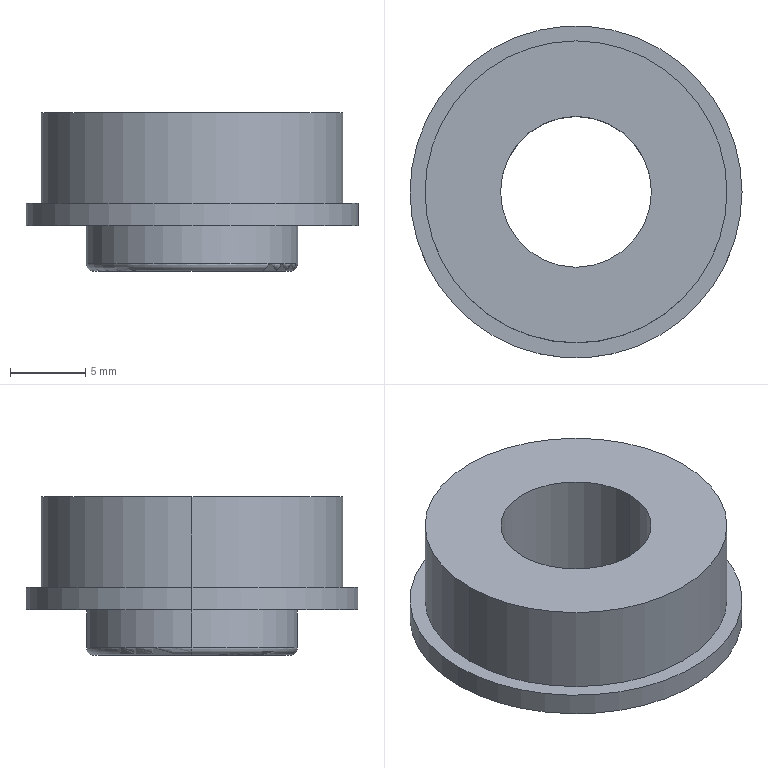Part | 1 solid | 14 faces | box 22 x 22 x 10.5 mm | volume 2090 mm3 | cylinder 8 | plane 4 | torus 2 | commonest cylinder face diameters 10 x2 14 x2 20 x2 22 x2
STEP:
#1=CARTESIAN_POINT('',(5.,0.,10.5));
#2=VERTEX_POINT('',#1);
#3=CARTESIAN_POINT('',(-5.,0.,10.5));
#4=VERTEX_POINT('',#3);
#5=CARTESIAN_POINT('',(0.,0.,10.5));
#6=DIRECTION('',(0.,0.,-1.));
#7=DIRECTION('',(-1.,0.,0.));
#8=AXIS2_PLACEMENT_3D('',#5,#6,#7);
#9=CIRCLE('',#8,5.);
#10=EDGE_CURVE('',#2,#4,#9,.T.);
#11=ORIENTED_EDGE('',*,*,#10,.F.);
#12=CARTESIAN_POINT('',(5.,0.,0.));
#13=VERTEX_POINT('',#12);
#14=CARTESIAN_POINT('',(5.,0.,10.5));
#15=DIRECTION('',(0.,0.,-1.));
#16=VECTOR('',#15,1000.);
#17=LINE('',#14,#16);
#18=EDGE_CURVE('',#2,#13,#17,.T.);
#19=ORIENTED_EDGE('',*,*,#18,.T.);
#20=CARTESIAN_POINT('',(-5.,0.,0.));
#21=VERTEX_POINT('',#20);
#22=CARTESIAN_POINT('',(0.,0.,0.));
#23=DIRECTION('',(0.,0.,-1.));
#24=DIRECTION('',(-1.,0.,0.));
#25=AXIS2_PLACEMENT_3D('',#22,#23,#24);
#26=CIRCLE('',#25,5.);
#27=EDGE_CURVE('',#13,#21,#26,.T.);
#28=ORIENTED_EDGE('',*,*,#27,.T.);
#29=CARTESIAN_POINT('',(-5.,0.,10.5));
#30=DIRECTION('',(0.,0.,-1.));
#31=VECTOR('',#30,1000.);
#32=LINE('',#29,#31);
#33=EDGE_CURVE('',#4,#21,#32,.T.);
#34=ORIENTED_EDGE('',*,*,#33,.F.);
#35=EDGE_LOOP('',(#11,#19,#28,#34));
#36=FACE_OUTER_BOUND('',#35,.T.);
#37=CARTESIAN_POINT('',(0.,0.,10.5));
#38=DIRECTION('',(0.,0.,-1.));
#39=DIRECTION('',(-1.,0.,0.));
#40=AXIS2_PLACEMENT_3D('',#37,#38,#39);
#41=CYLINDRICAL_SURFACE('',#40,5.);
#42=ADVANCED_FACE('',(#36),#41,.F.);
#43=CARTESIAN_POINT('',(-6.5,0.,0.));
#44=VERTEX_POINT('',#43);
#45=CARTESIAN_POINT('',(6.5,0.,0.));
#46=VERTEX_POINT('',#45);
#47=CARTESIAN_POINT('',(0.,0.,0.));
#48=DIRECTION('',(0.,0.,-1.));
#49=DIRECTION('',(1.,0.,0.));
#50=AXIS2_PLACEMENT_3D('',#47,#48,#49);
#51=CIRCLE('',#50,6.5);
#52=EDGE_CURVE('',#44,#46,#51,.T.);
#53=ORIENTED_EDGE('',*,*,#52,.F.);
#54=CARTESIAN_POINT('',(-7.,0.,0.5));
#55=VERTEX_POINT('',#54);
#56=CARTESIAN_POINT('',(-6.5,0.,0.5));
#57=DIRECTION('',(0.,1.,0.));
#58=DIRECTION('',(-1.,0.,0.));
#59=AXIS2_PLACEMENT_3D('',#56,#57,#58);
#60=CIRCLE('',#59,0.5);
#61=EDGE_CURVE('',#44,#55,#60,.T.);
#62=ORIENTED_EDGE('',*,*,#61,.T.);
#63=CARTESIAN_POINT('',(7.,0.,0.5));
#64=VERTEX_POINT('',#63);
#65=CARTESIAN_POINT('',(0.,0.,0.5));
#66=DIRECTION('',(0.,0.,1.));
#67=DIRECTION('',(1.,0.,0.));
#68=AXIS2_PLACEMENT_3D('',#65,#66,#67);
#69=CIRCLE('',#68,7.);
#70=EDGE_CURVE('',#64,#55,#69,.T.);
#71=ORIENTED_EDGE('',*,*,#70,.F.);
#72=CARTESIAN_POINT('',(6.5,0.,0.5));
#73=DIRECTION('',(0.,-1.,0.));
#74=DIRECTION('',(0.,0.,-1.));
#75=AXIS2_PLACEMENT_3D('',#72,#73,#74);
#76=CIRCLE('',#75,0.5);
#77=EDGE_CURVE('',#46,#64,#76,.T.);
#78=ORIENTED_EDGE('',*,*,#77,.F.);
#79=EDGE_LOOP('',(#53,#62,#71,#78));
#80=FACE_OUTER_BOUND('',#79,.T.);
#81=CARTESIAN_POINT('',(0.,0.,0.5));
#82=DIRECTION('',(0.,0.,1.));
#83=DIRECTION('',(1.,0.,0.));
#84=AXIS2_PLACEMENT_3D('',#81,#82,#83);
#85=TOROIDAL_SURFACE('',#84,6.5,0.5);
#86=ADVANCED_FACE('',(#80),#85,.T.);
#87=CARTESIAN_POINT('',(10.,0.,10.5));
#88=VERTEX_POINT('',#87);
#89=CARTESIAN_POINT('',(-10.,0.,10.5));
#90=VERTEX_POINT('',#89);
#91=CARTESIAN_POINT('',(0.,0.,10.5));
#92=DIRECTION('',(0.,0.,1.));
#93=DIRECTION('',(1.,0.,0.));
#94=AXIS2_PLACEMENT_3D('',#91,#92,#93);
#95=CIRCLE('',#94,10.);
#96=EDGE_CURVE('',#88,#90,#95,.T.);
#97=ORIENTED_EDGE('',*,*,#96,.F.);
#98=CARTESIAN_POINT('',(10.,0.,4.5));
#99=VERTEX_POINT('',#98);
#100=CARTESIAN_POINT('',(10.,0.,10.5));
#101=DIRECTION('',(0.,0.,-1.));
#102=VECTOR('',#101,1000.);
#103=LINE('',#100,#102);
#104=EDGE_CURVE('',#88,#99,#103,.T.);
#105=ORIENTED_EDGE('',*,*,#104,.T.);
#106=CARTESIAN_POINT('',(-10.,0.,4.5));
#107=VERTEX_POINT('',#106);
#108=CARTESIAN_POINT('',(0.,0.,4.5));
#109=DIRECTION('',(0.,0.,1.));
#110=DIRECTION('',(1.,0.,0.));
#111=AXIS2_PLACEMENT_3D('',#108,#109,#110);
#112=CIRCLE('',#111,10.);
#113=EDGE_CURVE('',#99,#107,#112,.T.);
#114=ORIENTED_EDGE('',*,*,#113,.T.);
#115=CARTESIAN_POINT('',(-10.,0.,10.5));
#116=DIRECTION('',(0.,0.,-1.));
#117=VECTOR('',#116,1000.);
#118=LINE('',#115,#117);
#119=EDGE_CURVE('',#90,#107,#118,.T.);
#120=ORIENTED_EDGE('',*,*,#119,.F.);
#121=EDGE_LOOP('',(#97,#105,#114,#120));
#122=FACE_OUTER_BOUND('',#121,.T.);
#123=CARTESIAN_POINT('',(0.,0.,10.5));
#124=DIRECTION('',(0.,0.,-1.));
#125=DIRECTION('',(-1.,0.,0.));
#126=AXIS2_PLACEMENT_3D('',#123,#124,#125);
#127=CYLINDRICAL_SURFACE('',#126,10.);
#128=ADVANCED_FACE('',(#122),#127,.T.);
#129=CARTESIAN_POINT('',(11.,0.,4.5));
#130=VERTEX_POINT('',#129);
#131=CARTESIAN_POINT('',(-11.,0.,4.5));
#132=VERTEX_POINT('',#131);
#133=CARTESIAN_POINT('',(0.,0.,4.5));
#134=DIRECTION('',(0.,0.,1.));
#135=DIRECTION('',(1.,0.,0.));
#136=AXIS2_PLACEMENT_3D('',#133,#134,#135);
#137=CIRCLE('',#136,11.);
#138=EDGE_CURVE('',#130,#132,#137,.T.);
#139=ORIENTED_EDGE('',*,*,#138,.F.);
#140=CARTESIAN_POINT('',(11.,0.,3.));
#141=VERTEX_POINT('',#140);
#142=CARTESIAN_POINT('',(11.,0.,4.5));
#143=DIRECTION('',(0.,0.,-1.));
#144=VECTOR('',#143,1000.);
#145=LINE('',#142,#144);
#146=EDGE_CURVE('',#130,#141,#145,.T.);
#147=ORIENTED_EDGE('',*,*,#146,.T.);
#148=CARTESIAN_POINT('',(-11.,0.,3.));
#149=VERTEX_POINT('',#148);
#150=CARTESIAN_POINT('',(0.,0.,3.));
#151=DIRECTION('',(0.,0.,1.));
#152=DIRECTION('',(1.,0.,0.));
#153=AXIS2_PLACEMENT_3D('',#150,#151,#152);
#154=CIRCLE('',#153,11.);
#155=EDGE_CURVE('',#141,#149,#154,.T.);
#156=ORIENTED_EDGE('',*,*,#155,.T.);
#157=CARTESIAN_POINT('',(-11.,0.,4.5));
#158=DIRECTION('',(0.,0.,-1.));
#159=VECTOR('',#158,1000.);
#160=LINE('',#157,#159);
#161=EDGE_CURVE('',#132,#149,#160,.T.);
#162=ORIENTED_EDGE('',*,*,#161,.F.);
#163=EDGE_LOOP('',(#139,#147,#156,#162));
#164=FACE_OUTER_BOUND('',#163,.T.);
#165=CARTESIAN_POINT('',(0.,0.,4.5));
#166=DIRECTION('',(0.,0.,-1.));
#167=DIRECTION('',(-1.,0.,0.));
#168=AXIS2_PLACEMENT_3D('',#165,#166,#167);
#169=CYLINDRICAL_SURFACE('',#168,11.);
#170=ADVANCED_FACE('',(#164),#169,.T.);
#171=CARTESIAN_POINT('',(7.,0.,3.));
#172=VERTEX_POINT('',#171);
#173=CARTESIAN_POINT('',(-7.,0.,3.));
#174=VERTEX_POINT('',#173);
#175=CARTESIAN_POINT('',(0.,0.,3.));
#176=DIRECTION('',(0.,0.,1.));
#177=DIRECTION('',(1.,0.,0.));
#178=AXIS2_PLACEMENT_3D('',#175,#176,#177);
#179=CIRCLE('',#178,7.);
#180=EDGE_CURVE('',#172,#174,#179,.T.);
#181=ORIENTED_EDGE('',*,*,#180,.F.);
#182=CARTESIAN_POINT('',(7.,0.,3.));
#183=DIRECTION('',(0.,0.,-1.));
#184=VECTOR('',#183,1000.);
#185=LINE('',#182,#184);
#186=EDGE_CURVE('',#172,#64,#185,.T.);
#187=ORIENTED_EDGE('',*,*,#186,.T.);
#188=ORIENTED_EDGE('',*,*,#70,.T.);
#189=CARTESIAN_POINT('',(-7.,0.,3.));
#190=DIRECTION('',(0.,0.,-1.));
#191=VECTOR('',#190,1000.);
#192=LINE('',#189,#191);
#193=EDGE_CURVE('',#174,#55,#192,.T.);
#194=ORIENTED_EDGE('',*,*,#193,.F.);
#195=EDGE_LOOP('',(#181,#187,#188,#194));
#196=FACE_OUTER_BOUND('',#195,.T.);
#197=CARTESIAN_POINT('',(0.,0.,3.));
#198=DIRECTION('',(0.,0.,-1.));
#199=DIRECTION('',(-1.,0.,0.));
#200=AXIS2_PLACEMENT_3D('',#197,#198,#199);
#201=CYLINDRICAL_SURFACE('',#200,7.);
#202=ADVANCED_FACE('',(#196),#201,.T.);
#203=ORIENTED_EDGE('',*,*,#186,.F.);
#204=CARTESIAN_POINT('',(0.,0.,3.));
#205=DIRECTION('',(0.,0.,1.));
#206=DIRECTION('',(1.,0.,0.));
#207=AXIS2_PLACEMENT_3D('',#204,#205,#206);
#208=CIRCLE('',#207,7.);
#209=EDGE_CURVE('',#174,#172,#208,.T.);
#210=ORIENTED_EDGE('',*,*,#209,.F.);
#211=ORIENTED_EDGE('',*,*,#193,.T.);
#212=CARTESIAN_POINT('',(0.,0.,0.5));
#213=DIRECTION('',(0.,0.,1.));
#214=DIRECTION('',(1.,0.,0.));
#215=AXIS2_PLACEMENT_3D('',#212,#213,#214);
#216=CIRCLE('',#215,7.);
#217=EDGE_CURVE('',#55,#64,#216,.T.);
#218=ORIENTED_EDGE('',*,*,#217,.T.);
#219=EDGE_LOOP('',(#203,#210,#211,#218));
#220=FACE_OUTER_BOUND('',#219,.T.);
#221=CARTESIAN_POINT('',(0.,0.,3.));
#222=DIRECTION('',(0.,0.,-1.));
#223=DIRECTION('',(-1.,0.,0.));
#224=AXIS2_PLACEMENT_3D('',#221,#222,#223);
#225=CYLINDRICAL_SURFACE('',#224,7.);
#226=ADVANCED_FACE('',(#220),#225,.T.);
#227=CARTESIAN_POINT('',(0.,0.,0.));
#228=DIRECTION('',(0.,0.,-1.));
#229=DIRECTION('',(1.,0.,0.));
#230=AXIS2_PLACEMENT_3D('',#227,#228,#229);
#231=CIRCLE('',#230,6.5);
#232=EDGE_CURVE('',#46,#44,#231,.T.);
#233=ORIENTED_EDGE('',*,*,#232,.T.);
#234=ORIENTED_EDGE('',*,*,#52,.T.);
#235=EDGE_LOOP('',(#233,#234));
#236=FACE_OUTER_BOUND('',#235,.T.);
#237=CARTESIAN_POINT('',(0.,0.,0.));
#238=DIRECTION('',(0.,0.,-1.));
#239=DIRECTION('',(-1.,0.,0.));
#240=AXIS2_PLACEMENT_3D('',#237,#238,#239);
#241=CIRCLE('',#240,5.);
#242=EDGE_CURVE('',#21,#13,#241,.T.);
#243=ORIENTED_EDGE('',*,*,#242,.F.);
#244=ORIENTED_EDGE('',*,*,#27,.F.);
#245=EDGE_LOOP('',(#243,#244));
#246=FACE_BOUND('',#245,.T.);
#247=CARTESIAN_POINT('',(0.,0.,0.));
#248=DIRECTION('',(0.,0.,1.));
#249=DIRECTION('',(1.,0.,0.));
#250=AXIS2_PLACEMENT_3D('',#247,#248,#249);
#251=PLANE('',#250);
#252=ADVANCED_FACE('',(#236,#246),#251,.F.);
#253=ORIENTED_EDGE('',*,*,#146,.F.);
#254=CARTESIAN_POINT('',(0.,0.,4.5));
#255=DIRECTION('',(0.,0.,1.));
#256=DIRECTION('',(1.,0.,0.));
#257=AXIS2_PLACEMENT_3D('',#254,#255,#256);
#258=CIRCLE('',#257,11.);
#259=EDGE_CURVE('',#132,#130,#258,.T.);
#260=ORIENTED_EDGE('',*,*,#259,.F.);
#261=ORIENTED_EDGE('',*,*,#161,.T.);
#262=CARTESIAN_POINT('',(0.,0.,3.));
#263=DIRECTION('',(0.,0.,1.));
#264=DIRECTION('',(1.,0.,0.));
#265=AXIS2_PLACEMENT_3D('',#262,#263,#264);
#266=CIRCLE('',#265,11.);
#267=EDGE_CURVE('',#149,#141,#266,.T.);
#268=ORIENTED_EDGE('',*,*,#267,.T.);
#269=EDGE_LOOP('',(#253,#260,#261,#268));
#270=FACE_OUTER_BOUND('',#269,.T.);
#271=CARTESIAN_POINT('',(0.,0.,4.5));
#272=DIRECTION('',(0.,0.,-1.));
#273=DIRECTION('',(-1.,0.,0.));
#274=AXIS2_PLACEMENT_3D('',#271,#272,#273);
#275=CYLINDRICAL_SURFACE('',#274,11.);
#276=ADVANCED_FACE('',(#270),#275,.T.);
#277=ORIENTED_EDGE('',*,*,#259,.T.);
#278=ORIENTED_EDGE('',*,*,#138,.T.);
#279=EDGE_LOOP('',(#277,#278));
#280=FACE_OUTER_BOUND('',#279,.T.);
#281=CARTESIAN_POINT('',(0.,0.,4.5));
#282=DIRECTION('',(0.,0.,1.));
#283=DIRECTION('',(1.,0.,0.));
#284=AXIS2_PLACEMENT_3D('',#281,#282,#283);
#285=CIRCLE('',#284,10.);
#286=EDGE_CURVE('',#107,#99,#285,.T.);
#287=ORIENTED_EDGE('',*,*,#286,.F.);
#288=ORIENTED_EDGE('',*,*,#113,.F.);
#289=EDGE_LOOP('',(#287,#288));
#290=FACE_BOUND('',#289,.T.);
#291=CARTESIAN_POINT('',(0.,0.,4.5));
#292=DIRECTION('',(0.,0.,1.));
#293=DIRECTION('',(1.,0.,0.));
#294=AXIS2_PLACEMENT_3D('',#291,#292,#293);
#295=PLANE('',#294);
#296=ADVANCED_FACE('',(#280,#290),#295,.T.);
#297=ORIENTED_EDGE('',*,*,#267,.F.);
#298=ORIENTED_EDGE('',*,*,#155,.F.);
#299=EDGE_LOOP('',(#297,#298));
#300=FACE_OUTER_BOUND('',#299,.T.);
#301=ORIENTED_EDGE('',*,*,#209,.T.);
#302=ORIENTED_EDGE('',*,*,#180,.T.);
#303=EDGE_LOOP('',(#301,#302));
#304=FACE_BOUND('',#303,.T.);
#305=CARTESIAN_POINT('',(0.,0.,3.));
#306=DIRECTION('',(0.,0.,1.));
#307=DIRECTION('',(1.,0.,0.));
#308=AXIS2_PLACEMENT_3D('',#305,#306,#307);
#309=PLANE('',#308);
#310=ADVANCED_FACE('',(#300,#304),#309,.F.);
#311=ORIENTED_EDGE('',*,*,#104,.F.);
#312=CARTESIAN_POINT('',(0.,0.,10.5));
#313=DIRECTION('',(0.,0.,1.));
#314=DIRECTION('',(1.,0.,0.));
#315=AXIS2_PLACEMENT_3D('',#312,#313,#314);
#316=CIRCLE('',#315,10.);
#317=EDGE_CURVE('',#90,#88,#316,.T.);
#318=ORIENTED_EDGE('',*,*,#317,.F.);
#319=ORIENTED_EDGE('',*,*,#119,.T.);
#320=ORIENTED_EDGE('',*,*,#286,.T.);
#321=EDGE_LOOP('',(#311,#318,#319,#320));
#322=FACE_OUTER_BOUND('',#321,.T.);
#323=CARTESIAN_POINT('',(0.,0.,10.5));
#324=DIRECTION('',(0.,0.,-1.));
#325=DIRECTION('',(-1.,0.,0.));
#326=AXIS2_PLACEMENT_3D('',#323,#324,#325);
#327=CYLINDRICAL_SURFACE('',#326,10.);
#328=ADVANCED_FACE('',(#322),#327,.T.);
#329=ORIENTED_EDGE('',*,*,#317,.T.);
#330=ORIENTED_EDGE('',*,*,#96,.T.);
#331=EDGE_LOOP('',(#329,#330));
#332=FACE_OUTER_BOUND('',#331,.T.);
#333=CARTESIAN_POINT('',(0.,0.,10.5));
#334=DIRECTION('',(0.,0.,-1.));
#335=DIRECTION('',(-1.,0.,0.));
#336=AXIS2_PLACEMENT_3D('',#333,#334,#335);
#337=CIRCLE('',#336,5.);
#338=EDGE_CURVE('',#4,#2,#337,.T.);
#339=ORIENTED_EDGE('',*,*,#338,.T.);
#340=ORIENTED_EDGE('',*,*,#10,.T.);
#341=EDGE_LOOP('',(#339,#340));
#342=FACE_BOUND('',#341,.T.);
#343=CARTESIAN_POINT('',(0.,0.,10.5));
#344=DIRECTION('',(0.,0.,1.));
#345=DIRECTION('',(1.,0.,0.));
#346=AXIS2_PLACEMENT_3D('',#343,#344,#345);
#347=PLANE('',#346);
#348=ADVANCED_FACE('',(#332,#342),#347,.T.);
#349=ORIENTED_EDGE('',*,*,#61,.F.);
#350=ORIENTED_EDGE('',*,*,#232,.F.);
#351=ORIENTED_EDGE('',*,*,#77,.T.);
#352=ORIENTED_EDGE('',*,*,#217,.F.);
#353=EDGE_LOOP('',(#349,#350,#351,#352));
#354=FACE_OUTER_BOUND('',#353,.T.);
#355=CARTESIAN_POINT('',(0.,0.,0.5));
#356=DIRECTION('',(0.,0.,1.));
#357=DIRECTION('',(1.,0.,0.));
#358=AXIS2_PLACEMENT_3D('',#355,#356,#357);
#359=TOROIDAL_SURFACE('',#358,6.5,0.5);
#360=ADVANCED_FACE('',(#354),#359,.T.);
#361=ORIENTED_EDGE('',*,*,#18,.F.);
#362=ORIENTED_EDGE('',*,*,#338,.F.);
#363=ORIENTED_EDGE('',*,*,#33,.T.);
#364=ORIENTED_EDGE('',*,*,#242,.T.);
#365=EDGE_LOOP('',(#361,#362,#363,#364));
#366=FACE_OUTER_BOUND('',#365,.T.);
#367=CARTESIAN_POINT('',(0.,0.,10.5));
#368=DIRECTION('',(0.,0.,-1.));
#369=DIRECTION('',(-1.,0.,0.));
#370=AXIS2_PLACEMENT_3D('',#367,#368,#369);
#371=CYLINDRICAL_SURFACE('',#370,5.);
#372=ADVANCED_FACE('',(#366),#371,.F.);
#373=CLOSED_SHELL('',(#42,#86,#128,#170,#202,#226,#252,#276,#296,#310,#328,#348,#360,#372));
#374=MANIFOLD_SOLID_BREP('',#373);
#375=CARTESIAN_POINT('',(0.,0.,0.));
#376=DIRECTION('',(0.,0.,1.));
#377=DIRECTION('',(1.,0.,0.));
#378=AXIS2_PLACEMENT_3D('',#375,#376,#377);
#379=(LENGTH_UNIT()NAMED_UNIT(*)SI_UNIT(.MILLI.,.METRE.));
#380=UNCERTAINTY_MEASURE_WITH_UNIT(LENGTH_MEASURE(0.00001),#379,'','');
#381=(NAMED_UNIT(*)PLANE_ANGLE_UNIT()SI_UNIT($,.RADIAN.));
#382=(NAMED_UNIT(*)SI_UNIT($,.STERADIAN.)SOLID_ANGLE_UNIT());
#383=(GEOMETRIC_REPRESENTATION_CONTEXT(3)GLOBAL_UNCERTAINTY_ASSIGNED_CONTEXT((#380))GLOBAL_UNIT_ASSIGNED_CONTEXT((#379,#381,#382))REPRESENTATION_CONTEXT('',''));
#384=ADVANCED_BREP_SHAPE_REPRESENTATION('',(#374,#378),#383);